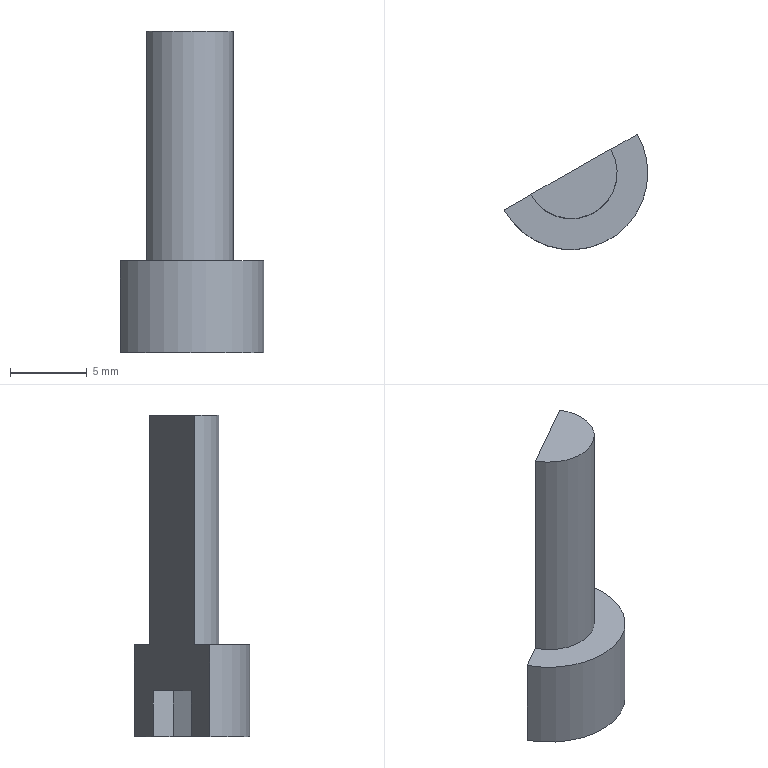Part | STEP file | LG M6_1.5F | 1 solid | 12 faces | box 9.384 x 7.531 x 21 mm | volume 424.771 mm3 | plane 9 | cylinder 3 | commonest cylinder face diameters 10 x2 6 x1
STEP:
#1=CARTESIAN_POINT('',(0.,0.,0.));
#2=DIRECTION('',(0.,0.,1.));
#3=DIRECTION('',(1.,0.,0.));
#4=AXIS2_PLACEMENT_3D('',#1,#2,#3);
#5=CARTESIAN_POINT('',(-4.384,-2.404,-6.));
#6=VERTEX_POINT('',#5);
#7=CARTESIAN_POINT('',(5.,0.,-6.));
#8=VERTEX_POINT('',#7);
#9=CARTESIAN_POINT('',(0.,0.,-6.));
#10=DIRECTION('',(0.,0.,1.));
#11=DIRECTION('',(1.,0.,0.));
#12=AXIS2_PLACEMENT_3D('',#9,#10,#11);
#13=CIRCLE('',#12,5.);
#14=CARTESIAN_POINT('',(0.,0.,-6.));
#15=DIRECTION('',(0.,0.,1.));
#16=DIRECTION('',(1.,0.,0.));
#17=AXIS2_PLACEMENT_3D('',#14,#15,#16);
#18=CYLINDRICAL_SURFACE('',#17,5.);
#19=CARTESIAN_POINT('',(0.,0.));
#20=DIRECTION('',(1.,0.));
#21=VECTOR('',#20,1.);
#22=LINE('',#19,#21);
#23=(GEOMETRIC_REPRESENTATION_CONTEXT(2)PARAMETRIC_REPRESENTATION_CONTEXT()REPRESENTATION_CONTEXT('',''));
#24=DEFINITIONAL_REPRESENTATION('',(#22),#23);
#25=PCURVE('',#18,#24);
#26=CARTESIAN_POINT('',(0.,0.,-6.));
#27=DIRECTION('',(0.,0.,1.));
#28=DIRECTION('',(1.,0.,0.));
#29=AXIS2_PLACEMENT_3D('',#26,#27,#28);
#30=PLANE('',#29);
#31=CARTESIAN_POINT('',(0.,0.));
#32=DIRECTION('',(1.,0.));
#33=AXIS2_PLACEMENT_2D('',#31,#32);
#34=CIRCLE('',#33,5.);
#35=(GEOMETRIC_REPRESENTATION_CONTEXT(2)PARAMETRIC_REPRESENTATION_CONTEXT()REPRESENTATION_CONTEXT('',''));
#36=DEFINITIONAL_REPRESENTATION('',(#34),#35);
#37=PCURVE('',#30,#36);
#38=SURFACE_CURVE('',#13,(#25,#37),.PCURVE_S1.);
#39=EDGE_CURVE('',#6,#8,#38,.T.);
#40=ORIENTED_EDGE('',*,*,#39,.T.);
#41=CARTESIAN_POINT('',(5.,0.,0.));
#42=VERTEX_POINT('',#41);
#43=CARTESIAN_POINT('',(5.,0.,-6.));
#44=DIRECTION('',(0.,0.,1.));
#45=VECTOR('',#44,1.);
#46=LINE('',#43,#45);
#47=CARTESIAN_POINT('',(6.283,0.));
#48=DIRECTION('',(0.,1.));
#49=VECTOR('',#48,1.);
#50=LINE('',#47,#49);
#51=(GEOMETRIC_REPRESENTATION_CONTEXT(2)PARAMETRIC_REPRESENTATION_CONTEXT()REPRESENTATION_CONTEXT('',''));
#52=DEFINITIONAL_REPRESENTATION('',(#50),#51);
#53=PCURVE('',#18,#52);
#54=CARTESIAN_POINT('',(0.,0.,-6.));
#55=DIRECTION('',(0.,0.,1.));
#56=DIRECTION('',(1.,0.,0.));
#57=AXIS2_PLACEMENT_3D('',#54,#55,#56);
#58=CYLINDRICAL_SURFACE('',#57,5.);
#59=CARTESIAN_POINT('',(0.,0.));
#60=DIRECTION('',(0.,1.));
#61=VECTOR('',#60,1.);
#62=LINE('',#59,#61);
#63=(GEOMETRIC_REPRESENTATION_CONTEXT(2)PARAMETRIC_REPRESENTATION_CONTEXT()REPRESENTATION_CONTEXT('',''));
#64=DEFINITIONAL_REPRESENTATION('',(#62),#63);
#65=PCURVE('',#58,#64);
#66=SURFACE_CURVE('',#46,(#53,#65),.PCURVE_S1.);
#67=EDGE_CURVE('',#8,#42,#66,.T.);
#68=ORIENTED_EDGE('',*,*,#67,.T.);
#69=CARTESIAN_POINT('',(-4.384,-2.404,0.));
#70=VERTEX_POINT('',#69);
#71=CARTESIAN_POINT('',(0.,0.,0.));
#72=DIRECTION('',(0.,0.,1.));
#73=DIRECTION('',(1.,0.,0.));
#74=AXIS2_PLACEMENT_3D('',#71,#72,#73);
#75=CIRCLE('',#74,5.);
#76=CARTESIAN_POINT('',(0.,6.));
#77=DIRECTION('',(1.,0.));
#78=VECTOR('',#77,1.);
#79=LINE('',#76,#78);
#80=(GEOMETRIC_REPRESENTATION_CONTEXT(2)PARAMETRIC_REPRESENTATION_CONTEXT()REPRESENTATION_CONTEXT('',''));
#81=DEFINITIONAL_REPRESENTATION('',(#79),#80);
#82=PCURVE('',#18,#81);
#83=CARTESIAN_POINT('',(0.,0.,0.));
#84=DIRECTION('',(0.,0.,1.));
#85=DIRECTION('',(1.,0.,0.));
#86=AXIS2_PLACEMENT_3D('',#83,#84,#85);
#87=PLANE('',#86);
#88=CARTESIAN_POINT('',(0.,0.));
#89=DIRECTION('',(1.,0.));
#90=AXIS2_PLACEMENT_2D('',#88,#89);
#91=CIRCLE('',#90,5.);
#92=(GEOMETRIC_REPRESENTATION_CONTEXT(2)PARAMETRIC_REPRESENTATION_CONTEXT()REPRESENTATION_CONTEXT('',''));
#93=DEFINITIONAL_REPRESENTATION('',(#91),#92);
#94=PCURVE('',#87,#93);
#95=SURFACE_CURVE('',#75,(#82,#94),.PCURVE_S1.);
#96=EDGE_CURVE('',#70,#42,#95,.T.);
#97=ORIENTED_EDGE('',*,*,#96,.F.);
#98=CARTESIAN_POINT('',(-4.384,-2.404,-6.));
#99=DIRECTION('',(0.,0.,1.));
#100=VECTOR('',#99,1.);
#101=LINE('',#98,#100);
#102=CARTESIAN_POINT('',(3.643,0.));
#103=DIRECTION('',(0.,1.));
#104=VECTOR('',#103,1.);
#105=LINE('',#102,#104);
#106=(GEOMETRIC_REPRESENTATION_CONTEXT(2)PARAMETRIC_REPRESENTATION_CONTEXT()REPRESENTATION_CONTEXT('',''));
#107=DEFINITIONAL_REPRESENTATION('',(#105),#106);
#108=PCURVE('',#18,#107);
#109=CARTESIAN_POINT('',(52.338,29.788,-18.57));
#110=DIRECTION('',(0.4936,-0.8697,0.));
#111=DIRECTION('',(0.8697,0.4936,0.));
#112=AXIS2_PLACEMENT_3D('',#109,#110,#111);
#113=PLANE('',#112);
#114=CARTESIAN_POINT('',(-65.221,12.57));
#115=DIRECTION('',(0.,1.));
#116=VECTOR('',#115,1.);
#117=LINE('',#114,#116);
#118=(GEOMETRIC_REPRESENTATION_CONTEXT(2)PARAMETRIC_REPRESENTATION_CONTEXT()REPRESENTATION_CONTEXT('',''));
#119=DEFINITIONAL_REPRESENTATION('',(#117),#118);
#120=PCURVE('',#113,#119);
#121=SURFACE_CURVE('',#101,(#108,#120),.PCURVE_S1.);
#122=EDGE_CURVE('',#6,#70,#121,.T.);
#123=ORIENTED_EDGE('',*,*,#122,.F.);
#124=EDGE_LOOP('',(#40,#68,#97,#123));
#125=FACE_BOUND('',#124,.T.);
#126=ADVANCED_FACE('',(#125),#18,.T.);
#127=CARTESIAN_POINT('',(-2.644,-1.417,0.));
#128=VERTEX_POINT('',#127);
#129=CARTESIAN_POINT('',(-0.03596,0.06336,0.));
#130=DIRECTION('',(0.8697,0.4936,0.));
#131=VECTOR('',#130,1.);
#132=LINE('',#129,#131);
#133=CARTESIAN_POINT('',(-0.03596,0.06336));
#134=DIRECTION('',(0.8697,0.4936));
#135=VECTOR('',#134,1.);
#136=LINE('',#133,#135);
#137=(GEOMETRIC_REPRESENTATION_CONTEXT(2)PARAMETRIC_REPRESENTATION_CONTEXT()REPRESENTATION_CONTEXT('',''));
#138=DEFINITIONAL_REPRESENTATION('',(#136),#137);
#139=PCURVE('',#87,#138);
#140=CARTESIAN_POINT('',(-60.221,18.57));
#141=DIRECTION('',(1.,0.));
#142=VECTOR('',#141,1.);
#143=LINE('',#140,#142);
#144=(GEOMETRIC_REPRESENTATION_CONTEXT(2)PARAMETRIC_REPRESENTATION_CONTEXT()REPRESENTATION_CONTEXT('',''));
#145=DEFINITIONAL_REPRESENTATION('',(#143),#144);
#146=PCURVE('',#113,#145);
#147=SURFACE_CURVE('',#132,(#139,#146),.PCURVE_S1.);
#148=EDGE_CURVE('',#70,#128,#147,.T.);
#149=ORIENTED_EDGE('',*,*,#148,.F.);
#150=ORIENTED_EDGE('',*,*,#96,.T.);
#151=CARTESIAN_POINT('',(4.312,2.531,0.));
#152=VERTEX_POINT('',#151);
#153=CARTESIAN_POINT('',(0.,0.,0.));
#154=DIRECTION('',(0.,0.,1.));
#155=DIRECTION('',(1.,0.,0.));
#156=AXIS2_PLACEMENT_3D('',#153,#154,#155);
#157=CIRCLE('',#156,5.);
#158=CARTESIAN_POINT('',(0.,0.));
#159=DIRECTION('',(1.,0.));
#160=AXIS2_PLACEMENT_2D('',#158,#159);
#161=CIRCLE('',#160,5.);
#162=(GEOMETRIC_REPRESENTATION_CONTEXT(2)PARAMETRIC_REPRESENTATION_CONTEXT()REPRESENTATION_CONTEXT('',''));
#163=DEFINITIONAL_REPRESENTATION('',(#161),#162);
#164=PCURVE('',#87,#163);
#165=CARTESIAN_POINT('',(0.,6.));
#166=DIRECTION('',(1.,0.));
#167=VECTOR('',#166,1.);
#168=LINE('',#165,#167);
#169=(GEOMETRIC_REPRESENTATION_CONTEXT(2)PARAMETRIC_REPRESENTATION_CONTEXT()REPRESENTATION_CONTEXT('',''));
#170=DEFINITIONAL_REPRESENTATION('',(#168),#169);
#171=PCURVE('',#58,#170);
#172=SURFACE_CURVE('',#157,(#164,#171),.PCURVE_S1.);
#173=EDGE_CURVE('',#42,#152,#172,.T.);
#174=ORIENTED_EDGE('',*,*,#173,.T.);
#175=CARTESIAN_POINT('',(2.572,1.544,0.));
#176=VERTEX_POINT('',#175);
#177=CARTESIAN_POINT('',(-0.03596,0.06336,0.));
#178=DIRECTION('',(0.8697,0.4936,0.));
#179=VECTOR('',#178,1.);
#180=LINE('',#177,#179);
#181=CARTESIAN_POINT('',(-0.03596,0.06336));
#182=DIRECTION('',(0.8697,0.4936));
#183=VECTOR('',#182,1.);
#184=LINE('',#181,#183);
#185=(GEOMETRIC_REPRESENTATION_CONTEXT(2)PARAMETRIC_REPRESENTATION_CONTEXT()REPRESENTATION_CONTEXT('',''));
#186=DEFINITIONAL_REPRESENTATION('',(#184),#185);
#187=PCURVE('',#87,#186);
#188=CARTESIAN_POINT('',(-60.221,18.57));
#189=DIRECTION('',(1.,0.));
#190=VECTOR('',#189,1.);
#191=LINE('',#188,#190);
#192=(GEOMETRIC_REPRESENTATION_CONTEXT(2)PARAMETRIC_REPRESENTATION_CONTEXT()REPRESENTATION_CONTEXT('',''));
#193=DEFINITIONAL_REPRESENTATION('',(#191),#192);
#194=PCURVE('',#113,#193);
#195=SURFACE_CURVE('',#180,(#187,#194),.PCURVE_S1.);
#196=EDGE_CURVE('',#176,#152,#195,.T.);
#197=ORIENTED_EDGE('',*,*,#196,.F.);
#198=CARTESIAN_POINT('',(0.,0.,0.));
#199=DIRECTION('',(0.,0.,1.));
#200=DIRECTION('',(1.,0.,0.));
#201=AXIS2_PLACEMENT_3D('',#198,#199,#200);
#202=CIRCLE('',#201,3.);
#203=CARTESIAN_POINT('',(0.,0.));
#204=DIRECTION('',(1.,0.));
#205=AXIS2_PLACEMENT_2D('',#203,#204);
#206=CIRCLE('',#205,3.);
#207=(GEOMETRIC_REPRESENTATION_CONTEXT(2)PARAMETRIC_REPRESENTATION_CONTEXT()REPRESENTATION_CONTEXT('',''));
#208=DEFINITIONAL_REPRESENTATION('',(#206),#207);
#209=PCURVE('',#87,#208);
#210=CARTESIAN_POINT('',(0.,0.,15.));
#211=DIRECTION('',(0.,0.,-1.));
#212=DIRECTION('',(-1.,0.,0.));
#213=AXIS2_PLACEMENT_3D('',#210,#211,#212);
#214=CYLINDRICAL_SURFACE('',#213,3.);
#215=CARTESIAN_POINT('',(9.425,15.));
#216=DIRECTION('',(-1.,0.));
#217=VECTOR('',#216,1.);
#218=LINE('',#215,#217);
#219=(GEOMETRIC_REPRESENTATION_CONTEXT(2)PARAMETRIC_REPRESENTATION_CONTEXT()REPRESENTATION_CONTEXT('',''));
#220=DEFINITIONAL_REPRESENTATION('',(#218),#219);
#221=PCURVE('',#214,#220);
#222=SURFACE_CURVE('',#202,(#209,#221),.PCURVE_S1.);
#223=EDGE_CURVE('',#128,#176,#222,.T.);
#224=ORIENTED_EDGE('',*,*,#223,.F.);
#225=EDGE_LOOP('',(#149,#150,#174,#197,#224));
#226=FACE_BOUND('',#225,.T.);
#227=ADVANCED_FACE('',(#226),#87,.T.);
#228=ORIENTED_EDGE('',*,*,#67,.F.);
#229=CARTESIAN_POINT('',(4.312,2.531,-6.));
#230=VERTEX_POINT('',#229);
#231=CARTESIAN_POINT('',(0.,0.,-6.));
#232=DIRECTION('',(0.,0.,1.));
#233=DIRECTION('',(1.,0.,0.));
#234=AXIS2_PLACEMENT_3D('',#231,#232,#233);
#235=CIRCLE('',#234,5.);
#236=CARTESIAN_POINT('',(0.,0.));
#237=DIRECTION('',(1.,0.));
#238=VECTOR('',#237,1.);
#239=LINE('',#236,#238);
#240=(GEOMETRIC_REPRESENTATION_CONTEXT(2)PARAMETRIC_REPRESENTATION_CONTEXT()REPRESENTATION_CONTEXT('',''));
#241=DEFINITIONAL_REPRESENTATION('',(#239),#240);
#242=PCURVE('',#58,#241);
#243=CARTESIAN_POINT('',(0.,0.));
#244=DIRECTION('',(1.,0.));
#245=AXIS2_PLACEMENT_2D('',#243,#244);
#246=CIRCLE('',#245,5.);
#247=(GEOMETRIC_REPRESENTATION_CONTEXT(2)PARAMETRIC_REPRESENTATION_CONTEXT()REPRESENTATION_CONTEXT('',''));
#248=DEFINITIONAL_REPRESENTATION('',(#246),#247);
#249=PCURVE('',#30,#248);
#250=SURFACE_CURVE('',#235,(#242,#249),.PCURVE_S1.);
#251=EDGE_CURVE('',#8,#230,#250,.T.);
#252=ORIENTED_EDGE('',*,*,#251,.T.);
#253=CARTESIAN_POINT('',(4.312,2.531,-6.));
#254=DIRECTION('',(0.,0.,-1.));
#255=VECTOR('',#254,1.);
#256=LINE('',#253,#255);
#257=CARTESIAN_POINT('',(0.5308,0.));
#258=DIRECTION('',(0.,-1.));
#259=VECTOR('',#258,1.);
#260=LINE('',#257,#259);
#261=(GEOMETRIC_REPRESENTATION_CONTEXT(2)PARAMETRIC_REPRESENTATION_CONTEXT()REPRESENTATION_CONTEXT('',''));
#262=DEFINITIONAL_REPRESENTATION('',(#260),#261);
#263=PCURVE('',#58,#262);
#264=CARTESIAN_POINT('',(-55.222,12.57));
#265=DIRECTION('',(0.,-1.));
#266=VECTOR('',#265,1.);
#267=LINE('',#264,#266);
#268=(GEOMETRIC_REPRESENTATION_CONTEXT(2)PARAMETRIC_REPRESENTATION_CONTEXT()REPRESENTATION_CONTEXT('',''));
#269=DEFINITIONAL_REPRESENTATION('',(#267),#268);
#270=PCURVE('',#113,#269);
#271=SURFACE_CURVE('',#256,(#263,#270),.PCURVE_S1.);
#272=EDGE_CURVE('',#152,#230,#271,.T.);
#273=ORIENTED_EDGE('',*,*,#272,.F.);
#274=ORIENTED_EDGE('',*,*,#173,.F.);
#275=EDGE_LOOP('',(#228,#252,#273,#274));
#276=FACE_BOUND('',#275,.T.);
#277=ADVANCED_FACE('',(#276),#58,.T.);
#278=ORIENTED_EDGE('',*,*,#39,.F.);
#279=CARTESIAN_POINT('',(-2.219,-1.176,-6.));
#280=VERTEX_POINT('',#279);
#281=CARTESIAN_POINT('',(-0.03596,0.06336,-6.));
#282=DIRECTION('',(0.8697,0.4936,0.));
#283=VECTOR('',#282,1.);
#284=LINE('',#281,#283);
#285=CARTESIAN_POINT('',(-0.03596,0.06336));
#286=DIRECTION('',(0.8697,0.4936));
#287=VECTOR('',#286,1.);
#288=LINE('',#285,#287);
#289=(GEOMETRIC_REPRESENTATION_CONTEXT(2)PARAMETRIC_REPRESENTATION_CONTEXT()REPRESENTATION_CONTEXT('',''));
#290=DEFINITIONAL_REPRESENTATION('',(#288),#289);
#291=PCURVE('',#30,#290);
#292=CARTESIAN_POINT('',(-60.221,12.57));
#293=DIRECTION('',(1.,0.));
#294=VECTOR('',#293,1.);
#295=LINE('',#292,#294);
#296=(GEOMETRIC_REPRESENTATION_CONTEXT(2)PARAMETRIC_REPRESENTATION_CONTEXT()REPRESENTATION_CONTEXT('',''));
#297=DEFINITIONAL_REPRESENTATION('',(#295),#296);
#298=PCURVE('',#113,#297);
#299=SURFACE_CURVE('',#284,(#291,#298),.PCURVE_S1.);
#300=EDGE_CURVE('',#6,#280,#299,.T.);
#301=ORIENTED_EDGE('',*,*,#300,.T.);
#302=CARTESIAN_POINT('',(-1.449,-2.51,-6.));
#303=VERTEX_POINT('',#302);
#304=CARTESIAN_POINT('',(-1.449,-2.51,-6.));
#305=DIRECTION('',(-0.5,0.866,0.));
#306=VECTOR('',#305,1.);
#307=LINE('',#304,#306);
#308=CARTESIAN_POINT('',(-1.449,-2.51));
#309=DIRECTION('',(-0.5,0.866));
#310=VECTOR('',#309,1.);
#311=LINE('',#308,#310);
#312=(GEOMETRIC_REPRESENTATION_CONTEXT(2)PARAMETRIC_REPRESENTATION_CONTEXT()REPRESENTATION_CONTEXT('',''));
#313=DEFINITIONAL_REPRESENTATION('',(#311),#312);
#314=PCURVE('',#30,#313);
#315=CARTESIAN_POINT('',(-1.449,-2.51,-3.));
#316=DIRECTION('',(-0.866,-0.5,0.));
#317=DIRECTION('',(0.5,-0.866,0.));
#318=AXIS2_PLACEMENT_3D('',#315,#316,#317);
#319=PLANE('',#318);
#320=CARTESIAN_POINT('',(0.,-3.));
#321=DIRECTION('',(-1.,0.));
#322=VECTOR('',#321,1.);
#323=LINE('',#320,#322);
#324=(GEOMETRIC_REPRESENTATION_CONTEXT(2)PARAMETRIC_REPRESENTATION_CONTEXT()REPRESENTATION_CONTEXT('',''));
#325=DEFINITIONAL_REPRESENTATION('',(#323),#324);
#326=PCURVE('',#319,#325);
#327=SURFACE_CURVE('',#307,(#314,#326),.PCURVE_S1.);
#328=EDGE_CURVE('',#303,#280,#327,.T.);
#329=ORIENTED_EDGE('',*,*,#328,.F.);
#330=CARTESIAN_POINT('',(1.449,-2.51,-6.));
#331=VERTEX_POINT('',#330);
#332=CARTESIAN_POINT('',(1.449,-2.51,-6.));
#333=DIRECTION('',(-1.,0.,0.));
#334=VECTOR('',#333,1.);
#335=LINE('',#332,#334);
#336=CARTESIAN_POINT('',(1.449,-2.51));
#337=DIRECTION('',(-1.,0.));
#338=VECTOR('',#337,1.);
#339=LINE('',#336,#338);
#340=(GEOMETRIC_REPRESENTATION_CONTEXT(2)PARAMETRIC_REPRESENTATION_CONTEXT()REPRESENTATION_CONTEXT('',''));
#341=DEFINITIONAL_REPRESENTATION('',(#339),#340);
#342=PCURVE('',#30,#341);
#343=CARTESIAN_POINT('',(1.449,-2.51,-3.));
#344=DIRECTION('',(0.,-1.,0.));
#345=DIRECTION('',(0.,0.,-1.));
#346=AXIS2_PLACEMENT_3D('',#343,#344,#345);
#347=PLANE('',#346);
#348=CARTESIAN_POINT('',(3.,0.));
#349=DIRECTION('',(0.,-1.));
#350=VECTOR('',#349,1.);
#351=LINE('',#348,#350);
#352=(GEOMETRIC_REPRESENTATION_CONTEXT(2)PARAMETRIC_REPRESENTATION_CONTEXT()REPRESENTATION_CONTEXT('',''));
#353=DEFINITIONAL_REPRESENTATION('',(#351),#352);
#354=PCURVE('',#347,#353);
#355=SURFACE_CURVE('',#335,(#342,#354),.PCURVE_S1.);
#356=EDGE_CURVE('',#331,#303,#355,.T.);
#357=ORIENTED_EDGE('',*,*,#356,.F.);
#358=CARTESIAN_POINT('',(2.898,0.,-6.));
#359=VERTEX_POINT('',#358);
#360=CARTESIAN_POINT('',(2.898,0.,-6.));
#361=DIRECTION('',(-0.5,-0.866,0.));
#362=VECTOR('',#361,1.);
#363=LINE('',#360,#362);
#364=CARTESIAN_POINT('',(2.898,0.));
#365=DIRECTION('',(-0.5,-0.866));
#366=VECTOR('',#365,1.);
#367=LINE('',#364,#366);
#368=(GEOMETRIC_REPRESENTATION_CONTEXT(2)PARAMETRIC_REPRESENTATION_CONTEXT()REPRESENTATION_CONTEXT('',''));
#369=DEFINITIONAL_REPRESENTATION('',(#367),#368);
#370=PCURVE('',#30,#369);
#371=CARTESIAN_POINT('',(2.898,0.,-3.));
#372=DIRECTION('',(0.866,-0.5,0.));
#373=DIRECTION('',(0.5,0.866,0.));
#374=AXIS2_PLACEMENT_3D('',#371,#372,#373);
#375=PLANE('',#374);
#376=CARTESIAN_POINT('',(0.,-3.));
#377=DIRECTION('',(-1.,0.));
#378=VECTOR('',#377,1.);
#379=LINE('',#376,#378);
#380=(GEOMETRIC_REPRESENTATION_CONTEXT(2)PARAMETRIC_REPRESENTATION_CONTEXT()REPRESENTATION_CONTEXT('',''));
#381=DEFINITIONAL_REPRESENTATION('',(#379),#380);
#382=PCURVE('',#375,#381);
#383=SURFACE_CURVE('',#363,(#370,#382),.PCURVE_S1.);
#384=EDGE_CURVE('',#359,#331,#383,.T.);
#385=ORIENTED_EDGE('',*,*,#384,.F.);
#386=CARTESIAN_POINT('',(2.147,1.302,-6.));
#387=VERTEX_POINT('',#386);
#388=CARTESIAN_POINT('',(1.449,2.51,-6.));
#389=DIRECTION('',(0.5,-0.866,0.));
#390=VECTOR('',#389,1.);
#391=LINE('',#388,#390);
#392=CARTESIAN_POINT('',(1.449,2.51));
#393=DIRECTION('',(0.5,-0.866));
#394=VECTOR('',#393,1.);
#395=LINE('',#392,#394);
#396=(GEOMETRIC_REPRESENTATION_CONTEXT(2)PARAMETRIC_REPRESENTATION_CONTEXT()REPRESENTATION_CONTEXT('',''));
#397=DEFINITIONAL_REPRESENTATION('',(#395),#396);
#398=PCURVE('',#30,#397);
#399=CARTESIAN_POINT('',(1.449,2.51,-3.));
#400=DIRECTION('',(0.866,0.5,0.));
#401=DIRECTION('',(-0.5,0.866,0.));
#402=AXIS2_PLACEMENT_3D('',#399,#400,#401);
#403=PLANE('',#402);
#404=CARTESIAN_POINT('',(0.,-3.));
#405=DIRECTION('',(-1.,0.));
#406=VECTOR('',#405,1.);
#407=LINE('',#404,#406);
#408=(GEOMETRIC_REPRESENTATION_CONTEXT(2)PARAMETRIC_REPRESENTATION_CONTEXT()REPRESENTATION_CONTEXT('',''));
#409=DEFINITIONAL_REPRESENTATION('',(#407),#408);
#410=PCURVE('',#403,#409);
#411=SURFACE_CURVE('',#391,(#398,#410),.PCURVE_S1.);
#412=EDGE_CURVE('',#387,#359,#411,.T.);
#413=ORIENTED_EDGE('',*,*,#412,.F.);
#414=CARTESIAN_POINT('',(-0.03596,0.06336,-6.));
#415=DIRECTION('',(0.8697,0.4936,0.));
#416=VECTOR('',#415,1.);
#417=LINE('',#414,#416);
#418=CARTESIAN_POINT('',(-0.03596,0.06336));
#419=DIRECTION('',(0.8697,0.4936));
#420=VECTOR('',#419,1.);
#421=LINE('',#418,#420);
#422=(GEOMETRIC_REPRESENTATION_CONTEXT(2)PARAMETRIC_REPRESENTATION_CONTEXT()REPRESENTATION_CONTEXT('',''));
#423=DEFINITIONAL_REPRESENTATION('',(#421),#422);
#424=PCURVE('',#30,#423);
#425=CARTESIAN_POINT('',(-60.221,12.57));
#426=DIRECTION('',(1.,0.));
#427=VECTOR('',#426,1.);
#428=LINE('',#425,#427);
#429=(GEOMETRIC_REPRESENTATION_CONTEXT(2)PARAMETRIC_REPRESENTATION_CONTEXT()REPRESENTATION_CONTEXT('',''));
#430=DEFINITIONAL_REPRESENTATION('',(#428),#429);
#431=PCURVE('',#113,#430);
#432=SURFACE_CURVE('',#417,(#424,#431),.PCURVE_S1.);
#433=EDGE_CURVE('',#387,#230,#432,.T.);
#434=ORIENTED_EDGE('',*,*,#433,.T.);
#435=ORIENTED_EDGE('',*,*,#251,.F.);
#436=EDGE_LOOP('',(#278,#301,#329,#357,#385,#413,#434,#435));
#437=FACE_BOUND('',#436,.T.);
#438=ADVANCED_FACE('',(#437),#30,.F.);
#439=CARTESIAN_POINT('',(-2.644,-1.417,15.));
#440=VERTEX_POINT('',#439);
#441=CARTESIAN_POINT('',(2.572,1.544,15.));
#442=VERTEX_POINT('',#441);
#443=CARTESIAN_POINT('',(0.,0.,15.));
#444=DIRECTION('',(0.,0.,1.));
#445=DIRECTION('',(1.,0.,0.));
#446=AXIS2_PLACEMENT_3D('',#443,#444,#445);
#447=CIRCLE('',#446,3.);
#448=CARTESIAN_POINT('',(9.425,0.));
#449=DIRECTION('',(-1.,0.));
#450=VECTOR('',#449,1.);
#451=LINE('',#448,#450);
#452=(GEOMETRIC_REPRESENTATION_CONTEXT(2)PARAMETRIC_REPRESENTATION_CONTEXT()REPRESENTATION_CONTEXT('',''));
#453=DEFINITIONAL_REPRESENTATION('',(#451),#452);
#454=PCURVE('',#214,#453);
#455=CARTESIAN_POINT('',(0.,0.,15.));
#456=DIRECTION('',(0.,0.,1.));
#457=DIRECTION('',(1.,0.,0.));
#458=AXIS2_PLACEMENT_3D('',#455,#456,#457);
#459=PLANE('',#458);
#460=CARTESIAN_POINT('',(0.,0.));
#461=DIRECTION('',(1.,0.));
#462=AXIS2_PLACEMENT_2D('',#460,#461);
#463=CIRCLE('',#462,3.);
#464=(GEOMETRIC_REPRESENTATION_CONTEXT(2)PARAMETRIC_REPRESENTATION_CONTEXT()REPRESENTATION_CONTEXT('',''));
#465=DEFINITIONAL_REPRESENTATION('',(#463),#464);
#466=PCURVE('',#459,#465);
#467=SURFACE_CURVE('',#447,(#454,#466),.PCURVE_S1.);
#468=EDGE_CURVE('',#440,#442,#467,.T.);
#469=ORIENTED_EDGE('',*,*,#468,.F.);
#470=CARTESIAN_POINT('',(-2.644,-1.417,15.));
#471=DIRECTION('',(0.,0.,-1.));
#472=VECTOR('',#471,1.);
#473=LINE('',#470,#472);
#474=CARTESIAN_POINT('',(5.791,0.));
#475=DIRECTION('',(0.,1.));
#476=VECTOR('',#475,1.);
#477=LINE('',#474,#476);
#478=(GEOMETRIC_REPRESENTATION_CONTEXT(2)PARAMETRIC_REPRESENTATION_CONTEXT()REPRESENTATION_CONTEXT('',''));
#479=DEFINITIONAL_REPRESENTATION('',(#477),#478);
#480=PCURVE('',#214,#479);
#481=CARTESIAN_POINT('',(-63.221,33.57));
#482=DIRECTION('',(0.,-1.));
#483=VECTOR('',#482,1.);
#484=LINE('',#481,#483);
#485=(GEOMETRIC_REPRESENTATION_CONTEXT(2)PARAMETRIC_REPRESENTATION_CONTEXT()REPRESENTATION_CONTEXT('',''));
#486=DEFINITIONAL_REPRESENTATION('',(#484),#485);
#487=PCURVE('',#113,#486);
#488=SURFACE_CURVE('',#473,(#480,#487),.PCURVE_S1.);
#489=EDGE_CURVE('',#440,#128,#488,.T.);
#490=ORIENTED_EDGE('',*,*,#489,.T.);
#491=ORIENTED_EDGE('',*,*,#223,.T.);
#492=CARTESIAN_POINT('',(2.572,1.544,15.));
#493=DIRECTION('',(0.,0.,1.));
#494=VECTOR('',#493,1.);
#495=LINE('',#492,#494);
#496=CARTESIAN_POINT('',(2.601,0.));
#497=DIRECTION('',(0.,-1.));
#498=VECTOR('',#497,1.);
#499=LINE('',#496,#498);
#500=(GEOMETRIC_REPRESENTATION_CONTEXT(2)PARAMETRIC_REPRESENTATION_CONTEXT()REPRESENTATION_CONTEXT('',''));
#501=DEFINITIONAL_REPRESENTATION('',(#499),#500);
#502=PCURVE('',#214,#501);
#503=CARTESIAN_POINT('',(-57.222,33.57));
#504=DIRECTION('',(0.,1.));
#505=VECTOR('',#504,1.);
#506=LINE('',#503,#505);
#507=(GEOMETRIC_REPRESENTATION_CONTEXT(2)PARAMETRIC_REPRESENTATION_CONTEXT()REPRESENTATION_CONTEXT('',''));
#508=DEFINITIONAL_REPRESENTATION('',(#506),#507);
#509=PCURVE('',#113,#508);
#510=SURFACE_CURVE('',#495,(#502,#509),.PCURVE_S1.);
#511=EDGE_CURVE('',#176,#442,#510,.T.);
#512=ORIENTED_EDGE('',*,*,#511,.T.);
#513=EDGE_LOOP('',(#469,#490,#491,#512));
#514=FACE_BOUND('',#513,.T.);
#515=ADVANCED_FACE('',(#514),#214,.T.);
#516=CARTESIAN_POINT('',(-0.03596,0.06336,15.));
#517=DIRECTION('',(0.8697,0.4936,0.));
#518=VECTOR('',#517,1.);
#519=LINE('',#516,#518);
#520=CARTESIAN_POINT('',(-0.03596,0.06336));
#521=DIRECTION('',(0.8697,0.4936));
#522=VECTOR('',#521,1.);
#523=LINE('',#520,#522);
#524=(GEOMETRIC_REPRESENTATION_CONTEXT(2)PARAMETRIC_REPRESENTATION_CONTEXT()REPRESENTATION_CONTEXT('',''));
#525=DEFINITIONAL_REPRESENTATION('',(#523),#524);
#526=PCURVE('',#459,#525);
#527=CARTESIAN_POINT('',(-60.221,33.57));
#528=DIRECTION('',(1.,0.));
#529=VECTOR('',#528,1.);
#530=LINE('',#527,#529);
#531=(GEOMETRIC_REPRESENTATION_CONTEXT(2)PARAMETRIC_REPRESENTATION_CONTEXT()REPRESENTATION_CONTEXT('',''));
#532=DEFINITIONAL_REPRESENTATION('',(#530),#531);
#533=PCURVE('',#113,#532);
#534=SURFACE_CURVE('',#519,(#526,#533),.PCURVE_S1.);
#535=EDGE_CURVE('',#440,#442,#534,.T.);
#536=ORIENTED_EDGE('',*,*,#535,.F.);
#537=ORIENTED_EDGE('',*,*,#468,.T.);
#538=EDGE_LOOP('',(#536,#537));
#539=FACE_BOUND('',#538,.T.);
#540=ADVANCED_FACE('',(#539),#459,.T.);
#541=ORIENTED_EDGE('',*,*,#328,.T.);
#542=CARTESIAN_POINT('',(-2.219,-1.176,-3.));
#543=VERTEX_POINT('',#542);
#544=CARTESIAN_POINT('',(-2.219,-1.176,-3.));
#545=DIRECTION('',(0.,0.,1.));
#546=VECTOR('',#545,1.);
#547=LINE('',#544,#546);
#548=CARTESIAN_POINT('',(-1.541,0.));
#549=DIRECTION('',(0.,1.));
#550=VECTOR('',#549,1.);
#551=LINE('',#548,#550);
#552=(GEOMETRIC_REPRESENTATION_CONTEXT(2)PARAMETRIC_REPRESENTATION_CONTEXT()REPRESENTATION_CONTEXT('',''));
#553=DEFINITIONAL_REPRESENTATION('',(#551),#552);
#554=PCURVE('',#319,#553);
#555=CARTESIAN_POINT('',(-62.732,15.57));
#556=DIRECTION('',(0.,1.));
#557=VECTOR('',#556,1.);
#558=LINE('',#555,#557);
#559=(GEOMETRIC_REPRESENTATION_CONTEXT(2)PARAMETRIC_REPRESENTATION_CONTEXT()REPRESENTATION_CONTEXT('',''));
#560=DEFINITIONAL_REPRESENTATION('',(#558),#559);
#561=PCURVE('',#113,#560);
#562=SURFACE_CURVE('',#547,(#554,#561),.PCURVE_S1.);
#563=EDGE_CURVE('',#280,#543,#562,.T.);
#564=ORIENTED_EDGE('',*,*,#563,.T.);
#565=CARTESIAN_POINT('',(-1.449,-2.51,-3.));
#566=VERTEX_POINT('',#565);
#567=CARTESIAN_POINT('',(-1.449,-2.51,-3.));
#568=DIRECTION('',(-0.5,0.866,0.));
#569=VECTOR('',#568,1.);
#570=LINE('',#567,#569);
#571=CARTESIAN_POINT('',(0.,0.));
#572=DIRECTION('',(-1.,0.));
#573=VECTOR('',#572,1.);
#574=LINE('',#571,#573);
#575=(GEOMETRIC_REPRESENTATION_CONTEXT(2)PARAMETRIC_REPRESENTATION_CONTEXT()REPRESENTATION_CONTEXT('',''));
#576=DEFINITIONAL_REPRESENTATION('',(#574),#575);
#577=PCURVE('',#319,#576);
#578=CARTESIAN_POINT('',(0.,0.,-3.));
#579=DIRECTION('',(0.,0.,-1.));
#580=DIRECTION('',(-1.,0.,0.));
#581=AXIS2_PLACEMENT_3D('',#578,#579,#580);
#582=PLANE('',#581);
#583=CARTESIAN_POINT('',(1.449,-2.51));
#584=DIRECTION('',(0.5,0.866));
#585=VECTOR('',#584,1.);
#586=LINE('',#583,#585);
#587=(GEOMETRIC_REPRESENTATION_CONTEXT(2)PARAMETRIC_REPRESENTATION_CONTEXT()REPRESENTATION_CONTEXT('',''));
#588=DEFINITIONAL_REPRESENTATION('',(#586),#587);
#589=PCURVE('',#582,#588);
#590=SURFACE_CURVE('',#570,(#577,#589),.PCURVE_S1.);
#591=EDGE_CURVE('',#566,#543,#590,.T.);
#592=ORIENTED_EDGE('',*,*,#591,.F.);
#593=CARTESIAN_POINT('',(-1.449,-2.51,-3.));
#594=DIRECTION('',(0.,0.,-1.));
#595=VECTOR('',#594,1.);
#596=LINE('',#593,#595);
#597=CARTESIAN_POINT('',(0.,0.));
#598=DIRECTION('',(0.,-1.));
#599=VECTOR('',#598,1.);
#600=LINE('',#597,#599);
#601=(GEOMETRIC_REPRESENTATION_CONTEXT(2)PARAMETRIC_REPRESENTATION_CONTEXT()REPRESENTATION_CONTEXT('',''));
#602=DEFINITIONAL_REPRESENTATION('',(#600),#601);
#603=PCURVE('',#319,#602);
#604=CARTESIAN_POINT('',(0.,-2.898));
#605=DIRECTION('',(1.,0.));
#606=VECTOR('',#605,1.);
#607=LINE('',#604,#606);
#608=(GEOMETRIC_REPRESENTATION_CONTEXT(2)PARAMETRIC_REPRESENTATION_CONTEXT()REPRESENTATION_CONTEXT('',''));
#609=DEFINITIONAL_REPRESENTATION('',(#607),#608);
#610=PCURVE('',#347,#609);
#611=SURFACE_CURVE('',#596,(#603,#610),.PCURVE_S1.);
#612=EDGE_CURVE('',#566,#303,#611,.T.);
#613=ORIENTED_EDGE('',*,*,#612,.T.);
#614=EDGE_LOOP('',(#541,#564,#592,#613));
#615=FACE_BOUND('',#614,.T.);
#616=ADVANCED_FACE('',(#615),#319,.F.);
#617=ORIENTED_EDGE('',*,*,#356,.T.);
#618=ORIENTED_EDGE('',*,*,#612,.F.);
#619=CARTESIAN_POINT('',(1.449,-2.51,-3.));
#620=VERTEX_POINT('',#619);
#621=CARTESIAN_POINT('',(1.449,-2.51,-3.));
#622=DIRECTION('',(-1.,0.,0.));
#623=VECTOR('',#622,1.);
#624=LINE('',#621,#623);
#625=CARTESIAN_POINT('',(0.,0.));
#626=DIRECTION('',(0.,-1.));
#627=VECTOR('',#626,1.);
#628=LINE('',#625,#627);
#629=(GEOMETRIC_REPRESENTATION_CONTEXT(2)PARAMETRIC_REPRESENTATION_CONTEXT()REPRESENTATION_CONTEXT('',''));
#630=DEFINITIONAL_REPRESENTATION('',(#628),#629);
#631=PCURVE('',#347,#630);
#632=CARTESIAN_POINT('',(-1.449,-2.51));
#633=DIRECTION('',(1.,0.));
#634=VECTOR('',#633,1.);
#635=LINE('',#632,#634);
#636=(GEOMETRIC_REPRESENTATION_CONTEXT(2)PARAMETRIC_REPRESENTATION_CONTEXT()REPRESENTATION_CONTEXT('',''));
#637=DEFINITIONAL_REPRESENTATION('',(#635),#636);
#638=PCURVE('',#582,#637);
#639=SURFACE_CURVE('',#624,(#631,#638),.PCURVE_S1.);
#640=EDGE_CURVE('',#620,#566,#639,.T.);
#641=ORIENTED_EDGE('',*,*,#640,.F.);
#642=CARTESIAN_POINT('',(1.449,-2.51,-3.));
#643=DIRECTION('',(0.,0.,-1.));
#644=VECTOR('',#643,1.);
#645=LINE('',#642,#644);
#646=CARTESIAN_POINT('',(0.,0.));
#647=DIRECTION('',(1.,0.));
#648=VECTOR('',#647,1.);
#649=LINE('',#646,#648);
#650=(GEOMETRIC_REPRESENTATION_CONTEXT(2)PARAMETRIC_REPRESENTATION_CONTEXT()REPRESENTATION_CONTEXT('',''));
#651=DEFINITIONAL_REPRESENTATION('',(#649),#650);
#652=PCURVE('',#347,#651);
#653=CARTESIAN_POINT('',(-2.898,0.));
#654=DIRECTION('',(0.,-1.));
#655=VECTOR('',#654,1.);
#656=LINE('',#653,#655);
#657=(GEOMETRIC_REPRESENTATION_CONTEXT(2)PARAMETRIC_REPRESENTATION_CONTEXT()REPRESENTATION_CONTEXT('',''));
#658=DEFINITIONAL_REPRESENTATION('',(#656),#657);
#659=PCURVE('',#375,#658);
#660=SURFACE_CURVE('',#645,(#652,#659),.PCURVE_S1.);
#661=EDGE_CURVE('',#620,#331,#660,.T.);
#662=ORIENTED_EDGE('',*,*,#661,.T.);
#663=EDGE_LOOP('',(#617,#618,#641,#662));
#664=FACE_BOUND('',#663,.T.);
#665=ADVANCED_FACE('',(#664),#347,.F.);
#666=ORIENTED_EDGE('',*,*,#384,.T.);
#667=ORIENTED_EDGE('',*,*,#661,.F.);
#668=CARTESIAN_POINT('',(2.898,0.,-3.));
#669=VERTEX_POINT('',#668);
#670=CARTESIAN_POINT('',(2.898,0.,-3.));
#671=DIRECTION('',(-0.5,-0.866,0.));
#672=VECTOR('',#671,1.);
#673=LINE('',#670,#672);
#674=CARTESIAN_POINT('',(0.,0.));
#675=DIRECTION('',(-1.,0.));
#676=VECTOR('',#675,1.);
#677=LINE('',#674,#676);
#678=(GEOMETRIC_REPRESENTATION_CONTEXT(2)PARAMETRIC_REPRESENTATION_CONTEXT()REPRESENTATION_CONTEXT('',''));
#679=DEFINITIONAL_REPRESENTATION('',(#677),#678);
#680=PCURVE('',#375,#679);
#681=CARTESIAN_POINT('',(-2.898,0.));
#682=DIRECTION('',(0.5,-0.866));
#683=VECTOR('',#682,1.);
#684=LINE('',#681,#683);
#685=(GEOMETRIC_REPRESENTATION_CONTEXT(2)PARAMETRIC_REPRESENTATION_CONTEXT()REPRESENTATION_CONTEXT('',''));
#686=DEFINITIONAL_REPRESENTATION('',(#684),#685);
#687=PCURVE('',#582,#686);
#688=SURFACE_CURVE('',#673,(#680,#687),.PCURVE_S1.);
#689=EDGE_CURVE('',#669,#620,#688,.T.);
#690=ORIENTED_EDGE('',*,*,#689,.F.);
#691=CARTESIAN_POINT('',(2.898,0.,-3.));
#692=DIRECTION('',(0.,0.,-1.));
#693=VECTOR('',#692,1.);
#694=LINE('',#691,#693);
#695=CARTESIAN_POINT('',(0.,0.));
#696=DIRECTION('',(0.,-1.));
#697=VECTOR('',#696,1.);
#698=LINE('',#695,#697);
#699=(GEOMETRIC_REPRESENTATION_CONTEXT(2)PARAMETRIC_REPRESENTATION_CONTEXT()REPRESENTATION_CONTEXT('',''));
#700=DEFINITIONAL_REPRESENTATION('',(#698),#699);
#701=PCURVE('',#375,#700);
#702=CARTESIAN_POINT('',(-2.898,0.));
#703=DIRECTION('',(0.,-1.));
#704=VECTOR('',#703,1.);
#705=LINE('',#702,#704);
#706=(GEOMETRIC_REPRESENTATION_CONTEXT(2)PARAMETRIC_REPRESENTATION_CONTEXT()REPRESENTATION_CONTEXT('',''));
#707=DEFINITIONAL_REPRESENTATION('',(#705),#706);
#708=PCURVE('',#403,#707);
#709=SURFACE_CURVE('',#694,(#701,#708),.PCURVE_S1.);
#710=EDGE_CURVE('',#669,#359,#709,.T.);
#711=ORIENTED_EDGE('',*,*,#710,.T.);
#712=EDGE_LOOP('',(#666,#667,#690,#711));
#713=FACE_BOUND('',#712,.T.);
#714=ADVANCED_FACE('',(#713),#375,.F.);
#715=CARTESIAN_POINT('',(2.147,1.302,-3.));
#716=VERTEX_POINT('',#715);
#717=CARTESIAN_POINT('',(1.449,2.51,-3.));
#718=DIRECTION('',(0.5,-0.866,0.));
#719=VECTOR('',#718,1.);
#720=LINE('',#717,#719);
#721=CARTESIAN_POINT('',(0.,0.));
#722=DIRECTION('',(-1.,0.));
#723=VECTOR('',#722,1.);
#724=LINE('',#721,#723);
#725=(GEOMETRIC_REPRESENTATION_CONTEXT(2)PARAMETRIC_REPRESENTATION_CONTEXT()REPRESENTATION_CONTEXT('',''));
#726=DEFINITIONAL_REPRESENTATION('',(#724),#725);
#727=PCURVE('',#403,#726);
#728=CARTESIAN_POINT('',(-1.449,2.51));
#729=DIRECTION('',(-0.5,-0.866));
#730=VECTOR('',#729,1.);
#731=LINE('',#728,#730);
#732=(GEOMETRIC_REPRESENTATION_CONTEXT(2)PARAMETRIC_REPRESENTATION_CONTEXT()REPRESENTATION_CONTEXT('',''));
#733=DEFINITIONAL_REPRESENTATION('',(#731),#732);
#734=PCURVE('',#582,#733);
#735=SURFACE_CURVE('',#720,(#727,#734),.PCURVE_S1.);
#736=EDGE_CURVE('',#716,#669,#735,.T.);
#737=ORIENTED_EDGE('',*,*,#736,.F.);
#738=CARTESIAN_POINT('',(2.147,1.302,-3.));
#739=DIRECTION('',(0.,0.,-1.));
#740=VECTOR('',#739,1.);
#741=LINE('',#738,#740);
#742=CARTESIAN_POINT('',(-1.395,0.));
#743=DIRECTION('',(0.,-1.));
#744=VECTOR('',#743,1.);
#745=LINE('',#742,#744);
#746=(GEOMETRIC_REPRESENTATION_CONTEXT(2)PARAMETRIC_REPRESENTATION_CONTEXT()REPRESENTATION_CONTEXT('',''));
#747=DEFINITIONAL_REPRESENTATION('',(#745),#746);
#748=PCURVE('',#403,#747);
#749=CARTESIAN_POINT('',(-57.712,15.57));
#750=DIRECTION('',(0.,-1.));
#751=VECTOR('',#750,1.);
#752=LINE('',#749,#751);
#753=(GEOMETRIC_REPRESENTATION_CONTEXT(2)PARAMETRIC_REPRESENTATION_CONTEXT()REPRESENTATION_CONTEXT('',''));
#754=DEFINITIONAL_REPRESENTATION('',(#752),#753);
#755=PCURVE('',#113,#754);
#756=SURFACE_CURVE('',#741,(#748,#755),.PCURVE_S1.);
#757=EDGE_CURVE('',#716,#387,#756,.T.);
#758=ORIENTED_EDGE('',*,*,#757,.T.);
#759=ORIENTED_EDGE('',*,*,#412,.T.);
#760=ORIENTED_EDGE('',*,*,#710,.F.);
#761=EDGE_LOOP('',(#737,#758,#759,#760));
#762=FACE_BOUND('',#761,.T.);
#763=ADVANCED_FACE('',(#762),#403,.F.);
#764=CARTESIAN_POINT('',(-0.03596,0.06336,-3.));
#765=DIRECTION('',(-0.8697,-0.4936,0.));
#766=VECTOR('',#765,1.);
#767=LINE('',#764,#766);
#768=CARTESIAN_POINT('',(0.03596,0.06336));
#769=DIRECTION('',(0.8697,-0.4936));
#770=VECTOR('',#769,1.);
#771=LINE('',#768,#770);
#772=(GEOMETRIC_REPRESENTATION_CONTEXT(2)PARAMETRIC_REPRESENTATION_CONTEXT()REPRESENTATION_CONTEXT('',''));
#773=DEFINITIONAL_REPRESENTATION('',(#771),#772);
#774=PCURVE('',#582,#773);
#775=CARTESIAN_POINT('',(-60.221,15.57));
#776=DIRECTION('',(-1.,0.));
#777=VECTOR('',#776,1.);
#778=LINE('',#775,#777);
#779=(GEOMETRIC_REPRESENTATION_CONTEXT(2)PARAMETRIC_REPRESENTATION_CONTEXT()REPRESENTATION_CONTEXT('',''));
#780=DEFINITIONAL_REPRESENTATION('',(#778),#779);
#781=PCURVE('',#113,#780);
#782=SURFACE_CURVE('',#767,(#774,#781),.PCURVE_S1.);
#783=EDGE_CURVE('',#716,#543,#782,.T.);
#784=ORIENTED_EDGE('',*,*,#783,.F.);
#785=ORIENTED_EDGE('',*,*,#736,.T.);
#786=ORIENTED_EDGE('',*,*,#689,.T.);
#787=ORIENTED_EDGE('',*,*,#640,.T.);
#788=ORIENTED_EDGE('',*,*,#591,.T.);
#789=EDGE_LOOP('',(#784,#785,#786,#787,#788));
#790=FACE_BOUND('',#789,.T.);
#791=ADVANCED_FACE('',(#790),#582,.T.);
#792=ORIENTED_EDGE('',*,*,#535,.T.);
#793=ORIENTED_EDGE('',*,*,#511,.F.);
#794=ORIENTED_EDGE('',*,*,#196,.T.);
#795=ORIENTED_EDGE('',*,*,#272,.T.);
#796=ORIENTED_EDGE('',*,*,#433,.F.);
#797=ORIENTED_EDGE('',*,*,#757,.F.);
#798=ORIENTED_EDGE('',*,*,#783,.T.);
#799=ORIENTED_EDGE('',*,*,#563,.F.);
#800=ORIENTED_EDGE('',*,*,#300,.F.);
#801=ORIENTED_EDGE('',*,*,#122,.T.);
#802=ORIENTED_EDGE('',*,*,#148,.T.);
#803=ORIENTED_EDGE('',*,*,#489,.F.);
#804=EDGE_LOOP('',(#792,#793,#794,#795,#796,#797,#798,#799,#800,#801,#802,#803));
#805=FACE_BOUND('',#804,.T.);
#806=ADVANCED_FACE('',(#805),#113,.F.);
#807=CLOSED_SHELL('',(#126,#227,#277,#438,#515,#540,#616,#665,#714,#763,#791,#806));
#808=MANIFOLD_SOLID_BREP('',#807);
#809=(LENGTH_UNIT()NAMED_UNIT(*)SI_UNIT(.MILLI.,.METRE.));
#810=UNCERTAINTY_MEASURE_WITH_UNIT(LENGTH_MEASURE(0.0000001),#809,'','');
#811=(NAMED_UNIT(*)PLANE_ANGLE_UNIT()SI_UNIT($,.RADIAN.));
#812=(NAMED_UNIT(*)SI_UNIT($,.STERADIAN.)SOLID_ANGLE_UNIT());
#813=(GEOMETRIC_REPRESENTATION_CONTEXT(3)GLOBAL_UNCERTAINTY_ASSIGNED_CONTEXT((#810))GLOBAL_UNIT_ASSIGNED_CONTEXT((#809,#811,#812))REPRESENTATION_CONTEXT('',''));
#814=ADVANCED_BREP_SHAPE_REPRESENTATION('',(#4,#808),#813);